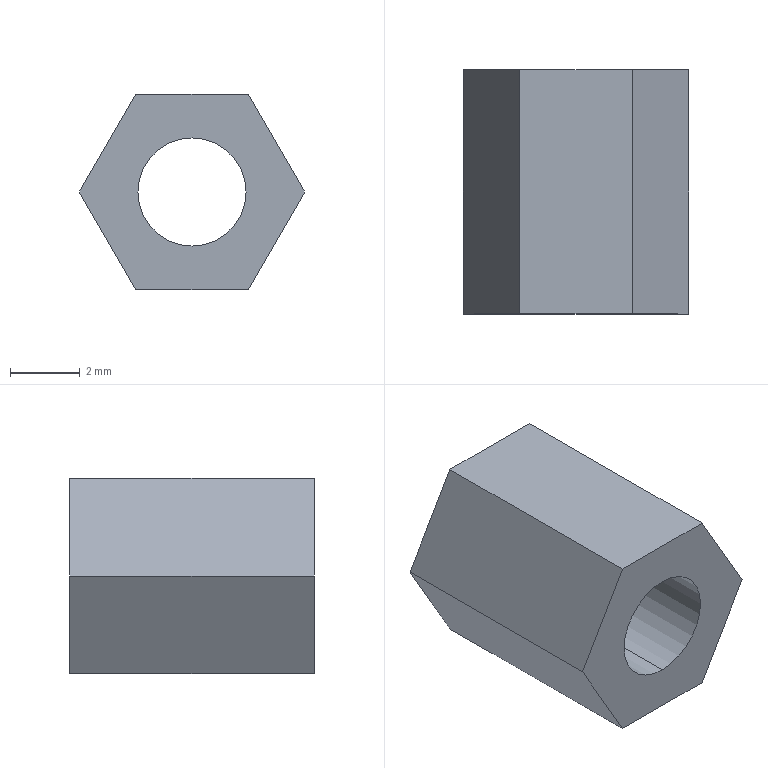Part | SolidWorks | features Extrusion 1 | 1 solid | 10 faces | box 6.466 x 7 x 5.6 mm | volume 137.276 mm3 | plane 8 | cylinder 2 | commonest cylinder face diameters 3.1 x2
STEP:
#1=CARTESIAN_POINT('',(0.,7.,-1.55));
#2=VERTEX_POINT('',#1);
#3=CARTESIAN_POINT('',(0.,7.,1.55));
#4=VERTEX_POINT('',#3);
#5=CARTESIAN_POINT('',(0.,7.,0.));
#6=DIRECTION('',(0.,1.,0.));
#7=DIRECTION('',(0.,0.,1.));
#8=AXIS2_PLACEMENT_3D('',#5,#6,#7);
#9=CIRCLE('',#8,1.55);
#10=EDGE_CURVE('',#2,#4,#9,.T.);
#11=ORIENTED_EDGE('',*,*,#10,.T.);
#12=CARTESIAN_POINT('',(0.,0.,1.55));
#13=VERTEX_POINT('',#12);
#14=CARTESIAN_POINT('',(0.,7.,1.55));
#15=DIRECTION('',(0.,-1.,0.));
#16=VECTOR('',#15,1000.);
#17=LINE('',#14,#16);
#18=EDGE_CURVE('',#4,#13,#17,.T.);
#19=ORIENTED_EDGE('',*,*,#18,.T.);
#20=CARTESIAN_POINT('',(0.,0.,-1.55));
#21=VERTEX_POINT('',#20);
#22=CARTESIAN_POINT('',(0.,0.,0.));
#23=DIRECTION('',(0.,1.,0.));
#24=DIRECTION('',(0.,0.,1.));
#25=AXIS2_PLACEMENT_3D('',#22,#23,#24);
#26=CIRCLE('',#25,1.55);
#27=EDGE_CURVE('',#21,#13,#26,.T.);
#28=ORIENTED_EDGE('',*,*,#27,.F.);
#29=CARTESIAN_POINT('',(0.,7.,-1.55));
#30=DIRECTION('',(0.,-1.,0.));
#31=VECTOR('',#30,1000.);
#32=LINE('',#29,#31);
#33=EDGE_CURVE('',#2,#21,#32,.T.);
#34=ORIENTED_EDGE('',*,*,#33,.F.);
#35=EDGE_LOOP('',(#11,#19,#28,#34));
#36=FACE_OUTER_BOUND('',#35,.T.);
#37=CARTESIAN_POINT('',(0.,7.,0.));
#38=DIRECTION('',(0.,-1.,0.));
#39=DIRECTION('',(0.,0.,-1.));
#40=AXIS2_PLACEMENT_3D('',#37,#38,#39);
#41=CYLINDRICAL_SURFACE('',#40,1.55);
#42=ADVANCED_FACE('',(#36),#41,.F.);
#43=CARTESIAN_POINT('',(-1.617,7.,2.8));
#44=VERTEX_POINT('',#43);
#45=CARTESIAN_POINT('',(1.617,7.,2.8));
#46=VERTEX_POINT('',#45);
#47=CARTESIAN_POINT('',(-1.617,7.,2.8));
#48=DIRECTION('',(1.,0.,0.));
#49=VECTOR('',#48,1000.);
#50=LINE('',#47,#49);
#51=EDGE_CURVE('',#44,#46,#50,.T.);
#52=ORIENTED_EDGE('',*,*,#51,.T.);
#53=CARTESIAN_POINT('',(3.233,7.,0.));
#54=VERTEX_POINT('',#53);
#55=CARTESIAN_POINT('',(1.617,7.,2.8));
#56=DIRECTION('',(0.5,0.,-0.866));
#57=VECTOR('',#56,1000.);
#58=LINE('',#55,#57);
#59=EDGE_CURVE('',#46,#54,#58,.T.);
#60=ORIENTED_EDGE('',*,*,#59,.T.);
#61=CARTESIAN_POINT('',(1.617,7.,-2.8));
#62=VERTEX_POINT('',#61);
#63=CARTESIAN_POINT('',(3.233,7.,0.));
#64=DIRECTION('',(-0.5,0.,-0.866));
#65=VECTOR('',#64,1000.);
#66=LINE('',#63,#65);
#67=EDGE_CURVE('',#54,#62,#66,.T.);
#68=ORIENTED_EDGE('',*,*,#67,.T.);
#69=CARTESIAN_POINT('',(-1.617,7.,-2.8));
#70=VERTEX_POINT('',#69);
#71=CARTESIAN_POINT('',(1.617,7.,-2.8));
#72=DIRECTION('',(-1.,0.,0.));
#73=VECTOR('',#72,1000.);
#74=LINE('',#71,#73);
#75=EDGE_CURVE('',#62,#70,#74,.T.);
#76=ORIENTED_EDGE('',*,*,#75,.T.);
#77=CARTESIAN_POINT('',(-3.233,7.,0.));
#78=VERTEX_POINT('',#77);
#79=CARTESIAN_POINT('',(-1.617,7.,-2.8));
#80=DIRECTION('',(-0.5,0.,0.866));
#81=VECTOR('',#80,1000.);
#82=LINE('',#79,#81);
#83=EDGE_CURVE('',#70,#78,#82,.T.);
#84=ORIENTED_EDGE('',*,*,#83,.T.);
#85=CARTESIAN_POINT('',(-3.233,7.,0.));
#86=DIRECTION('',(0.5,0.,0.866));
#87=VECTOR('',#86,1000.);
#88=LINE('',#85,#87);
#89=EDGE_CURVE('',#78,#44,#88,.T.);
#90=ORIENTED_EDGE('',*,*,#89,.T.);
#91=EDGE_LOOP('',(#52,#60,#68,#76,#84,#90));
#92=FACE_OUTER_BOUND('',#91,.T.);
#93=ORIENTED_EDGE('',*,*,#10,.F.);
#94=CARTESIAN_POINT('',(0.,7.,0.));
#95=DIRECTION('',(0.,1.,0.));
#96=DIRECTION('',(0.,0.,1.));
#97=AXIS2_PLACEMENT_3D('',#94,#95,#96);
#98=CIRCLE('',#97,1.55);
#99=EDGE_CURVE('',#4,#2,#98,.T.);
#100=ORIENTED_EDGE('',*,*,#99,.F.);
#101=EDGE_LOOP('',(#93,#100));
#102=FACE_BOUND('',#101,.T.);
#103=CARTESIAN_POINT('',(0.,7.,0.));
#104=DIRECTION('',(0.,1.,0.));
#105=DIRECTION('',(0.,0.,1.));
#106=AXIS2_PLACEMENT_3D('',#103,#104,#105);
#107=PLANE('',#106);
#108=ADVANCED_FACE('',(#92,#102),#107,.T.);
#109=CARTESIAN_POINT('',(-1.617,0.,2.8));
#110=VERTEX_POINT('',#109);
#111=CARTESIAN_POINT('',(1.617,0.,2.8));
#112=VERTEX_POINT('',#111);
#113=CARTESIAN_POINT('',(-1.617,0.,2.8));
#114=DIRECTION('',(1.,0.,0.));
#115=VECTOR('',#114,1000.);
#116=LINE('',#113,#115);
#117=EDGE_CURVE('',#110,#112,#116,.T.);
#118=ORIENTED_EDGE('',*,*,#117,.F.);
#119=CARTESIAN_POINT('',(-3.233,0.,0.));
#120=VERTEX_POINT('',#119);
#121=CARTESIAN_POINT('',(-3.233,0.,0.));
#122=DIRECTION('',(0.5,0.,0.866));
#123=VECTOR('',#122,1000.);
#124=LINE('',#121,#123);
#125=EDGE_CURVE('',#120,#110,#124,.T.);
#126=ORIENTED_EDGE('',*,*,#125,.F.);
#127=CARTESIAN_POINT('',(-1.617,0.,-2.8));
#128=VERTEX_POINT('',#127);
#129=CARTESIAN_POINT('',(-1.617,0.,-2.8));
#130=DIRECTION('',(-0.5,0.,0.866));
#131=VECTOR('',#130,1000.);
#132=LINE('',#129,#131);
#133=EDGE_CURVE('',#128,#120,#132,.T.);
#134=ORIENTED_EDGE('',*,*,#133,.F.);
#135=CARTESIAN_POINT('',(1.617,0.,-2.8));
#136=VERTEX_POINT('',#135);
#137=CARTESIAN_POINT('',(1.617,0.,-2.8));
#138=DIRECTION('',(-1.,0.,0.));
#139=VECTOR('',#138,1000.);
#140=LINE('',#137,#139);
#141=EDGE_CURVE('',#136,#128,#140,.T.);
#142=ORIENTED_EDGE('',*,*,#141,.F.);
#143=CARTESIAN_POINT('',(3.233,0.,0.));
#144=VERTEX_POINT('',#143);
#145=CARTESIAN_POINT('',(3.233,0.,0.));
#146=DIRECTION('',(-0.5,0.,-0.866));
#147=VECTOR('',#146,1000.);
#148=LINE('',#145,#147);
#149=EDGE_CURVE('',#144,#136,#148,.T.);
#150=ORIENTED_EDGE('',*,*,#149,.F.);
#151=CARTESIAN_POINT('',(1.617,0.,2.8));
#152=DIRECTION('',(0.5,0.,-0.866));
#153=VECTOR('',#152,1000.);
#154=LINE('',#151,#153);
#155=EDGE_CURVE('',#112,#144,#154,.T.);
#156=ORIENTED_EDGE('',*,*,#155,.F.);
#157=EDGE_LOOP('',(#118,#126,#134,#142,#150,#156));
#158=FACE_OUTER_BOUND('',#157,.T.);
#159=ORIENTED_EDGE('',*,*,#27,.T.);
#160=CARTESIAN_POINT('',(0.,0.,0.));
#161=DIRECTION('',(0.,1.,0.));
#162=DIRECTION('',(0.,0.,1.));
#163=AXIS2_PLACEMENT_3D('',#160,#161,#162);
#164=CIRCLE('',#163,1.55);
#165=EDGE_CURVE('',#13,#21,#164,.T.);
#166=ORIENTED_EDGE('',*,*,#165,.T.);
#167=EDGE_LOOP('',(#159,#166));
#168=FACE_BOUND('',#167,.T.);
#169=CARTESIAN_POINT('',(0.,0.,0.));
#170=DIRECTION('',(0.,1.,0.));
#171=DIRECTION('',(0.,0.,1.));
#172=AXIS2_PLACEMENT_3D('',#169,#170,#171);
#173=PLANE('',#172);
#174=ADVANCED_FACE('',(#158,#168),#173,.F.);
#175=ORIENTED_EDGE('',*,*,#117,.T.);
#176=CARTESIAN_POINT('',(1.617,7.,2.8));
#177=DIRECTION('',(0.,-1.,0.));
#178=VECTOR('',#177,1000.);
#179=LINE('',#176,#178);
#180=EDGE_CURVE('',#46,#112,#179,.T.);
#181=ORIENTED_EDGE('',*,*,#180,.F.);
#182=ORIENTED_EDGE('',*,*,#51,.F.);
#183=CARTESIAN_POINT('',(-1.617,7.,2.8));
#184=DIRECTION('',(0.,-1.,0.));
#185=VECTOR('',#184,1000.);
#186=LINE('',#183,#185);
#187=EDGE_CURVE('',#44,#110,#186,.T.);
#188=ORIENTED_EDGE('',*,*,#187,.T.);
#189=EDGE_LOOP('',(#175,#181,#182,#188));
#190=FACE_OUTER_BOUND('',#189,.T.);
#191=CARTESIAN_POINT('',(-1.617,7.,2.8));
#192=DIRECTION('',(0.,0.,-1.));
#193=DIRECTION('',(-1.,0.,0.));
#194=AXIS2_PLACEMENT_3D('',#191,#192,#193);
#195=PLANE('',#194);
#196=ADVANCED_FACE('',(#190),#195,.F.);
#197=ORIENTED_EDGE('',*,*,#155,.T.);
#198=CARTESIAN_POINT('',(3.233,7.,0.));
#199=DIRECTION('',(0.,-1.,0.));
#200=VECTOR('',#199,1000.);
#201=LINE('',#198,#200);
#202=EDGE_CURVE('',#54,#144,#201,.T.);
#203=ORIENTED_EDGE('',*,*,#202,.F.);
#204=ORIENTED_EDGE('',*,*,#59,.F.);
#205=ORIENTED_EDGE('',*,*,#180,.T.);
#206=EDGE_LOOP('',(#197,#203,#204,#205));
#207=FACE_OUTER_BOUND('',#206,.T.);
#208=CARTESIAN_POINT('',(1.617,7.,2.8));
#209=DIRECTION('',(-0.866,0.,-0.5));
#210=DIRECTION('',(-0.5,0.,0.866));
#211=AXIS2_PLACEMENT_3D('',#208,#209,#210);
#212=PLANE('',#211);
#213=ADVANCED_FACE('',(#207),#212,.F.);
#214=ORIENTED_EDGE('',*,*,#149,.T.);
#215=CARTESIAN_POINT('',(1.617,7.,-2.8));
#216=DIRECTION('',(0.,-1.,0.));
#217=VECTOR('',#216,1000.);
#218=LINE('',#215,#217);
#219=EDGE_CURVE('',#62,#136,#218,.T.);
#220=ORIENTED_EDGE('',*,*,#219,.F.);
#221=ORIENTED_EDGE('',*,*,#67,.F.);
#222=ORIENTED_EDGE('',*,*,#202,.T.);
#223=EDGE_LOOP('',(#214,#220,#221,#222));
#224=FACE_OUTER_BOUND('',#223,.T.);
#225=CARTESIAN_POINT('',(3.233,7.,0.));
#226=DIRECTION('',(-0.866,0.,0.5));
#227=DIRECTION('',(0.5,0.,0.866));
#228=AXIS2_PLACEMENT_3D('',#225,#226,#227);
#229=PLANE('',#228);
#230=ADVANCED_FACE('',(#224),#229,.F.);
#231=ORIENTED_EDGE('',*,*,#141,.T.);
#232=CARTESIAN_POINT('',(-1.617,7.,-2.8));
#233=DIRECTION('',(0.,-1.,0.));
#234=VECTOR('',#233,1000.);
#235=LINE('',#232,#234);
#236=EDGE_CURVE('',#70,#128,#235,.T.);
#237=ORIENTED_EDGE('',*,*,#236,.F.);
#238=ORIENTED_EDGE('',*,*,#75,.F.);
#239=ORIENTED_EDGE('',*,*,#219,.T.);
#240=EDGE_LOOP('',(#231,#237,#238,#239));
#241=FACE_OUTER_BOUND('',#240,.T.);
#242=CARTESIAN_POINT('',(1.617,7.,-2.8));
#243=DIRECTION('',(0.,0.,1.));
#244=DIRECTION('',(1.,0.,0.));
#245=AXIS2_PLACEMENT_3D('',#242,#243,#244);
#246=PLANE('',#245);
#247=ADVANCED_FACE('',(#241),#246,.F.);
#248=ORIENTED_EDGE('',*,*,#133,.T.);
#249=CARTESIAN_POINT('',(-3.233,7.,0.));
#250=DIRECTION('',(0.,-1.,0.));
#251=VECTOR('',#250,1000.);
#252=LINE('',#249,#251);
#253=EDGE_CURVE('',#78,#120,#252,.T.);
#254=ORIENTED_EDGE('',*,*,#253,.F.);
#255=ORIENTED_EDGE('',*,*,#83,.F.);
#256=ORIENTED_EDGE('',*,*,#236,.T.);
#257=EDGE_LOOP('',(#248,#254,#255,#256));
#258=FACE_OUTER_BOUND('',#257,.T.);
#259=CARTESIAN_POINT('',(-1.617,7.,-2.8));
#260=DIRECTION('',(0.866,0.,0.5));
#261=DIRECTION('',(0.5,0.,-0.866));
#262=AXIS2_PLACEMENT_3D('',#259,#260,#261);
#263=PLANE('',#262);
#264=ADVANCED_FACE('',(#258),#263,.F.);
#265=ORIENTED_EDGE('',*,*,#125,.T.);
#266=ORIENTED_EDGE('',*,*,#187,.F.);
#267=ORIENTED_EDGE('',*,*,#89,.F.);
#268=ORIENTED_EDGE('',*,*,#253,.T.);
#269=EDGE_LOOP('',(#265,#266,#267,#268));
#270=FACE_OUTER_BOUND('',#269,.T.);
#271=CARTESIAN_POINT('',(-3.233,7.,0.));
#272=DIRECTION('',(0.866,0.,-0.5));
#273=DIRECTION('',(-0.5,0.,-0.866));
#274=AXIS2_PLACEMENT_3D('',#271,#272,#273);
#275=PLANE('',#274);
#276=ADVANCED_FACE('',(#270),#275,.F.);
#277=ORIENTED_EDGE('',*,*,#18,.F.);
#278=ORIENTED_EDGE('',*,*,#99,.T.);
#279=ORIENTED_EDGE('',*,*,#33,.T.);
#280=ORIENTED_EDGE('',*,*,#165,.F.);
#281=EDGE_LOOP('',(#277,#278,#279,#280));
#282=FACE_OUTER_BOUND('',#281,.T.);
#283=CARTESIAN_POINT('',(0.,7.,0.));
#284=DIRECTION('',(0.,-1.,0.));
#285=DIRECTION('',(0.,0.,-1.));
#286=AXIS2_PLACEMENT_3D('',#283,#284,#285);
#287=CYLINDRICAL_SURFACE('',#286,1.55);
#288=ADVANCED_FACE('',(#282),#287,.F.);
#289=CLOSED_SHELL('',(#42,#108,#174,#196,#213,#230,#247,#264,#276,#288));
#290=MANIFOLD_SOLID_BREP('',#289);
#291=CARTESIAN_POINT('',(0.,0.,0.));
#292=DIRECTION('',(0.,0.,1.));
#293=DIRECTION('',(1.,0.,0.));
#294=AXIS2_PLACEMENT_3D('',#291,#292,#293);
#295=(LENGTH_UNIT()NAMED_UNIT(*)SI_UNIT(.MILLI.,.METRE.));
#296=UNCERTAINTY_MEASURE_WITH_UNIT(LENGTH_MEASURE(0.00001),#295,'','');
#297=(NAMED_UNIT(*)PLANE_ANGLE_UNIT()SI_UNIT($,.RADIAN.));
#298=(NAMED_UNIT(*)SI_UNIT($,.STERADIAN.)SOLID_ANGLE_UNIT());
#299=(GEOMETRIC_REPRESENTATION_CONTEXT(3)GLOBAL_UNCERTAINTY_ASSIGNED_CONTEXT((#296))GLOBAL_UNIT_ASSIGNED_CONTEXT((#295,#297,#298))REPRESENTATION_CONTEXT('',''));
#300=ADVANCED_BREP_SHAPE_REPRESENTATION('',(#290,#294),#299);